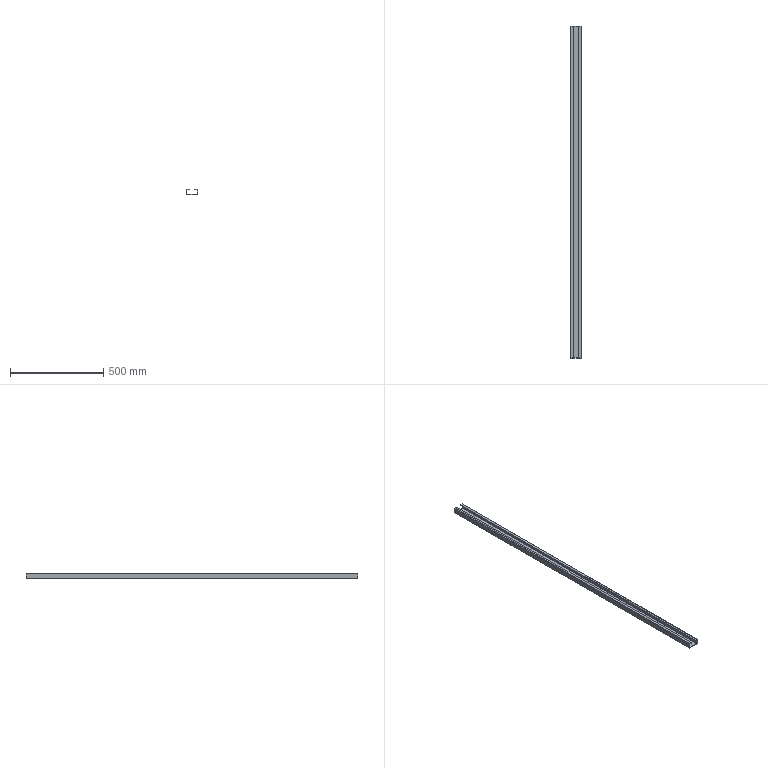Part | SolidWorks | features BaseBody 1 | 1 solid | 38 faces | box 60 x 1776 x 30 mm | volume 606457 mm3 | plane 30 | cylinder 8 | commonest cylinder face diameters 1.473 x4 6.473 x4
STEP:
#1=CARTESIAN_POINT('',(15.,888.,25.));
#2=VERTEX_POINT('',#1);
#3=CARTESIAN_POINT('',(15.,-888.,25.));
#4=VERTEX_POINT('',#3);
#5=CARTESIAN_POINT('',(15.,-888.,25.));
#6=DIRECTION('',(0.,-1.,0.));
#7=VECTOR('',#6,1000.);
#8=LINE('',#5,#7);
#9=EDGE_CURVE('',#2,#4,#8,.T.);
#10=ORIENTED_EDGE('',*,*,#9,.T.);
#11=CARTESIAN_POINT('',(15.,-888.,27.5));
#12=VERTEX_POINT('',#11);
#13=CARTESIAN_POINT('',(15.,-888.,27.5));
#14=DIRECTION('',(0.,0.,-1.));
#15=VECTOR('',#14,1000.);
#16=LINE('',#13,#15);
#17=EDGE_CURVE('',#12,#4,#16,.T.);
#18=ORIENTED_EDGE('',*,*,#17,.F.);
#19=CARTESIAN_POINT('',(15.,888.,27.5));
#20=VERTEX_POINT('',#19);
#21=CARTESIAN_POINT('',(15.,0.,27.5));
#22=DIRECTION('',(0.,-1.,0.));
#23=VECTOR('',#22,1000.);
#24=LINE('',#21,#23);
#25=EDGE_CURVE('',#20,#12,#24,.T.);
#26=ORIENTED_EDGE('',*,*,#25,.F.);
#27=CARTESIAN_POINT('',(15.,888.,27.5));
#28=DIRECTION('',(0.,0.,-1.));
#29=VECTOR('',#28,1000.);
#30=LINE('',#27,#29);
#31=EDGE_CURVE('',#20,#2,#30,.T.);
#32=ORIENTED_EDGE('',*,*,#31,.T.);
#33=EDGE_LOOP('',(#10,#18,#26,#32));
#34=FACE_OUTER_BOUND('',#33,.T.);
#35=CARTESIAN_POINT('',(15.,-888.,27.5));
#36=DIRECTION('',(1.,0.,0.));
#37=DIRECTION('',(0.,0.,-1.));
#38=AXIS2_PLACEMENT_3D('',#35,#36,#37);
#39=PLANE('',#38);
#40=ADVANCED_FACE('',(#34),#39,.F.);
#41=CARTESIAN_POINT('',(26.763,888.,25.));
#42=VERTEX_POINT('',#41);
#43=CARTESIAN_POINT('',(15.,888.,25.));
#44=DIRECTION('',(-1.,0.,0.));
#45=VECTOR('',#44,1000.);
#46=LINE('',#43,#45);
#47=EDGE_CURVE('',#42,#2,#46,.T.);
#48=ORIENTED_EDGE('',*,*,#47,.F.);
#49=CARTESIAN_POINT('',(26.763,-888.,25.));
#50=VERTEX_POINT('',#49);
#51=CARTESIAN_POINT('',(26.763,-888.,25.));
#52=DIRECTION('',(0.,1.,0.));
#53=VECTOR('',#52,1000.);
#54=LINE('',#51,#53);
#55=EDGE_CURVE('',#50,#42,#54,.T.);
#56=ORIENTED_EDGE('',*,*,#55,.F.);
#57=CARTESIAN_POINT('',(27.5,-888.,25.));
#58=DIRECTION('',(1.,0.,0.));
#59=VECTOR('',#58,1000.);
#60=LINE('',#57,#59);
#61=EDGE_CURVE('',#4,#50,#60,.T.);
#62=ORIENTED_EDGE('',*,*,#61,.F.);
#63=ORIENTED_EDGE('',*,*,#9,.F.);
#64=EDGE_LOOP('',(#48,#56,#62,#63));
#65=FACE_OUTER_BOUND('',#64,.T.);
#66=CARTESIAN_POINT('',(0.,0.,25.));
#67=DIRECTION('',(0.,0.,-1.));
#68=DIRECTION('',(-1.,0.,0.));
#69=AXIS2_PLACEMENT_3D('',#66,#67,#68);
#70=PLANE('',#69);
#71=ADVANCED_FACE('',(#65),#70,.T.);
#72=CARTESIAN_POINT('',(26.763,888.,27.5));
#73=VERTEX_POINT('',#72);
#74=CARTESIAN_POINT('',(26.763,-888.,27.5));
#75=VERTEX_POINT('',#74);
#76=CARTESIAN_POINT('',(26.763,-888.,27.5));
#77=DIRECTION('',(0.,-1.,0.));
#78=VECTOR('',#77,1000.);
#79=LINE('',#76,#78);
#80=EDGE_CURVE('',#73,#75,#79,.T.);
#81=ORIENTED_EDGE('',*,*,#80,.F.);
#82=CARTESIAN_POINT('',(0.,888.,27.5));
#83=DIRECTION('',(-1.,0.,0.));
#84=VECTOR('',#83,1000.);
#85=LINE('',#82,#84);
#86=EDGE_CURVE('',#73,#20,#85,.T.);
#87=ORIENTED_EDGE('',*,*,#86,.T.);
#88=ORIENTED_EDGE('',*,*,#25,.T.);
#89=CARTESIAN_POINT('',(0.,-888.,27.5));
#90=DIRECTION('',(1.,0.,0.));
#91=VECTOR('',#90,1000.);
#92=LINE('',#89,#91);
#93=EDGE_CURVE('',#12,#75,#92,.T.);
#94=ORIENTED_EDGE('',*,*,#93,.T.);
#95=EDGE_LOOP('',(#81,#87,#88,#94));
#96=FACE_OUTER_BOUND('',#95,.T.);
#97=CARTESIAN_POINT('',(0.,0.,27.5));
#98=DIRECTION('',(0.,0.,-1.));
#99=DIRECTION('',(-1.,0.,0.));
#100=AXIS2_PLACEMENT_3D('',#97,#98,#99);
#101=PLANE('',#100);
#102=ADVANCED_FACE('',(#96),#101,.F.);
#103=CARTESIAN_POINT('',(26.763,-888.,27.5));
#104=DIRECTION('',(0.,0.,1.));
#105=VECTOR('',#104,1000.);
#106=LINE('',#103,#105);
#107=EDGE_CURVE('',#50,#75,#106,.T.);
#108=ORIENTED_EDGE('',*,*,#107,.T.);
#109=ORIENTED_EDGE('',*,*,#93,.F.);
#110=ORIENTED_EDGE('',*,*,#17,.T.);
#111=ORIENTED_EDGE('',*,*,#61,.T.);
#112=EDGE_LOOP('',(#108,#109,#110,#111));
#113=FACE_OUTER_BOUND('',#112,.T.);
#114=CARTESIAN_POINT('',(27.5,-888.,27.5));
#115=DIRECTION('',(0.,1.,0.));
#116=DIRECTION('',(0.,0.,-1.));
#117=AXIS2_PLACEMENT_3D('',#114,#115,#116);
#118=PLANE('',#117);
#119=ADVANCED_FACE('',(#113),#118,.F.);
#120=CARTESIAN_POINT('',(26.763,888.,25.));
#121=DIRECTION('',(0.,0.,1.));
#122=VECTOR('',#121,1000.);
#123=LINE('',#120,#122);
#124=EDGE_CURVE('',#42,#73,#123,.T.);
#125=ORIENTED_EDGE('',*,*,#124,.F.);
#126=ORIENTED_EDGE('',*,*,#47,.T.);
#127=ORIENTED_EDGE('',*,*,#31,.F.);
#128=ORIENTED_EDGE('',*,*,#86,.F.);
#129=EDGE_LOOP('',(#125,#126,#127,#128));
#130=FACE_OUTER_BOUND('',#129,.T.);
#131=CARTESIAN_POINT('',(15.,888.,27.5));
#132=DIRECTION('',(0.,-1.,0.));
#133=DIRECTION('',(-1.,0.,0.));
#134=AXIS2_PLACEMENT_3D('',#131,#132,#133);
#135=PLANE('',#134);
#136=ADVANCED_FACE('',(#130),#135,.F.);
#137=CARTESIAN_POINT('',(27.5,888.,24.263));
#138=VERTEX_POINT('',#137);
#139=CARTESIAN_POINT('',(27.5,-888.,24.263));
#140=VERTEX_POINT('',#139);
#141=CARTESIAN_POINT('',(27.5,888.,24.263));
#142=DIRECTION('',(0.,-1.,0.));
#143=VECTOR('',#142,1000.);
#144=LINE('',#141,#143);
#145=EDGE_CURVE('',#138,#140,#144,.T.);
#146=ORIENTED_EDGE('',*,*,#145,.T.);
#147=CARTESIAN_POINT('',(26.763,-888.,24.263));
#148=DIRECTION('',(0.,-1.,0.));
#149=DIRECTION('',(0.,0.,1.));
#150=AXIS2_PLACEMENT_3D('',#147,#148,#149);
#151=CIRCLE('',#150,0.7366);
#152=EDGE_CURVE('',#140,#50,#151,.T.);
#153=ORIENTED_EDGE('',*,*,#152,.T.);
#154=ORIENTED_EDGE('',*,*,#55,.T.);
#155=CARTESIAN_POINT('',(26.763,888.,24.263));
#156=DIRECTION('',(0.,1.,0.));
#157=DIRECTION('',(0.,0.,1.));
#158=AXIS2_PLACEMENT_3D('',#155,#156,#157);
#159=CIRCLE('',#158,0.7366);
#160=EDGE_CURVE('',#42,#138,#159,.T.);
#161=ORIENTED_EDGE('',*,*,#160,.T.);
#162=EDGE_LOOP('',(#146,#153,#154,#161));
#163=FACE_OUTER_BOUND('',#162,.T.);
#164=CARTESIAN_POINT('',(26.763,888.,24.263));
#165=DIRECTION('',(0.,1.,0.));
#166=DIRECTION('',(0.,0.,1.));
#167=AXIS2_PLACEMENT_3D('',#164,#165,#166);
#168=CYLINDRICAL_SURFACE('',#167,0.7366);
#169=ADVANCED_FACE('',(#163),#168,.F.);
#170=CARTESIAN_POINT('',(30.,888.,24.263));
#171=VERTEX_POINT('',#170);
#172=CARTESIAN_POINT('',(30.,-888.,24.263));
#173=VERTEX_POINT('',#172);
#174=CARTESIAN_POINT('',(30.,888.,24.263));
#175=DIRECTION('',(0.,-1.,0.));
#176=VECTOR('',#175,1000.);
#177=LINE('',#174,#176);
#178=EDGE_CURVE('',#171,#173,#177,.T.);
#179=ORIENTED_EDGE('',*,*,#178,.F.);
#180=CARTESIAN_POINT('',(26.763,888.,24.263));
#181=DIRECTION('',(0.,1.,0.));
#182=DIRECTION('',(0.,0.,1.));
#183=AXIS2_PLACEMENT_3D('',#180,#181,#182);
#184=CIRCLE('',#183,3.237);
#185=EDGE_CURVE('',#73,#171,#184,.T.);
#186=ORIENTED_EDGE('',*,*,#185,.F.);
#187=ORIENTED_EDGE('',*,*,#80,.T.);
#188=CARTESIAN_POINT('',(26.763,-888.,24.263));
#189=DIRECTION('',(0.,-1.,0.));
#190=DIRECTION('',(0.,0.,1.));
#191=AXIS2_PLACEMENT_3D('',#188,#189,#190);
#192=CIRCLE('',#191,3.237);
#193=EDGE_CURVE('',#173,#75,#192,.T.);
#194=ORIENTED_EDGE('',*,*,#193,.F.);
#195=EDGE_LOOP('',(#179,#186,#187,#194));
#196=FACE_OUTER_BOUND('',#195,.T.);
#197=CARTESIAN_POINT('',(26.763,888.,24.263));
#198=DIRECTION('',(0.,1.,0.));
#199=DIRECTION('',(0.,0.,1.));
#200=AXIS2_PLACEMENT_3D('',#197,#198,#199);
#201=CYLINDRICAL_SURFACE('',#200,3.237);
#202=ADVANCED_FACE('',(#196),#201,.T.);
#203=ORIENTED_EDGE('',*,*,#160,.F.);
#204=ORIENTED_EDGE('',*,*,#124,.T.);
#205=ORIENTED_EDGE('',*,*,#185,.T.);
#206=CARTESIAN_POINT('',(27.5,888.,24.263));
#207=DIRECTION('',(1.,0.,0.));
#208=VECTOR('',#207,1000.);
#209=LINE('',#206,#208);
#210=EDGE_CURVE('',#138,#171,#209,.T.);
#211=ORIENTED_EDGE('',*,*,#210,.F.);
#212=EDGE_LOOP('',(#203,#204,#205,#211));
#213=FACE_OUTER_BOUND('',#212,.T.);
#214=CARTESIAN_POINT('',(26.763,888.,24.263));
#215=DIRECTION('',(0.,-1.,0.));
#216=DIRECTION('',(0.,0.,-1.));
#217=AXIS2_PLACEMENT_3D('',#214,#215,#216);
#218=PLANE('',#217);
#219=ADVANCED_FACE('',(#213),#218,.F.);
#220=ORIENTED_EDGE('',*,*,#107,.F.);
#221=ORIENTED_EDGE('',*,*,#152,.F.);
#222=CARTESIAN_POINT('',(27.5,-888.,24.263));
#223=DIRECTION('',(1.,0.,0.));
#224=VECTOR('',#223,1000.);
#225=LINE('',#222,#224);
#226=EDGE_CURVE('',#140,#173,#225,.T.);
#227=ORIENTED_EDGE('',*,*,#226,.T.);
#228=ORIENTED_EDGE('',*,*,#193,.T.);
#229=EDGE_LOOP('',(#220,#221,#227,#228));
#230=FACE_OUTER_BOUND('',#229,.T.);
#231=CARTESIAN_POINT('',(26.763,-888.,24.263));
#232=DIRECTION('',(0.,-1.,0.));
#233=DIRECTION('',(0.,0.,-1.));
#234=AXIS2_PLACEMENT_3D('',#231,#232,#233);
#235=PLANE('',#234);
#236=ADVANCED_FACE('',(#230),#235,.T.);
#237=CARTESIAN_POINT('',(-15.,-888.,25.));
#238=VERTEX_POINT('',#237);
#239=CARTESIAN_POINT('',(-15.,888.,25.));
#240=VERTEX_POINT('',#239);
#241=CARTESIAN_POINT('',(-15.,888.,25.));
#242=DIRECTION('',(0.,1.,0.));
#243=VECTOR('',#242,1000.);
#244=LINE('',#241,#243);
#245=EDGE_CURVE('',#238,#240,#244,.T.);
#246=ORIENTED_EDGE('',*,*,#245,.T.);
#247=CARTESIAN_POINT('',(-15.,888.,27.5));
#248=VERTEX_POINT('',#247);
#249=CARTESIAN_POINT('',(-15.,888.,27.5));
#250=DIRECTION('',(0.,0.,-1.));
#251=VECTOR('',#250,1000.);
#252=LINE('',#249,#251);
#253=EDGE_CURVE('',#248,#240,#252,.T.);
#254=ORIENTED_EDGE('',*,*,#253,.F.);
#255=CARTESIAN_POINT('',(-15.,-888.,27.5));
#256=VERTEX_POINT('',#255);
#257=CARTESIAN_POINT('',(-15.,0.,27.5));
#258=DIRECTION('',(0.,1.,0.));
#259=VECTOR('',#258,1000.);
#260=LINE('',#257,#259);
#261=EDGE_CURVE('',#256,#248,#260,.T.);
#262=ORIENTED_EDGE('',*,*,#261,.F.);
#263=CARTESIAN_POINT('',(-15.,-888.,27.5));
#264=DIRECTION('',(0.,0.,-1.));
#265=VECTOR('',#264,1000.);
#266=LINE('',#263,#265);
#267=EDGE_CURVE('',#256,#238,#266,.T.);
#268=ORIENTED_EDGE('',*,*,#267,.T.);
#269=EDGE_LOOP('',(#246,#254,#262,#268));
#270=FACE_OUTER_BOUND('',#269,.T.);
#271=CARTESIAN_POINT('',(-15.,888.,27.5));
#272=DIRECTION('',(-1.,0.,0.));
#273=DIRECTION('',(0.,0.,1.));
#274=AXIS2_PLACEMENT_3D('',#271,#272,#273);
#275=PLANE('',#274);
#276=ADVANCED_FACE('',(#270),#275,.F.);
#277=CARTESIAN_POINT('',(-26.763,-888.,25.));
#278=VERTEX_POINT('',#277);
#279=CARTESIAN_POINT('',(-15.,-888.,25.));
#280=DIRECTION('',(1.,0.,0.));
#281=VECTOR('',#280,1000.);
#282=LINE('',#279,#281);
#283=EDGE_CURVE('',#278,#238,#282,.T.);
#284=ORIENTED_EDGE('',*,*,#283,.F.);
#285=CARTESIAN_POINT('',(-26.763,888.,25.));
#286=VERTEX_POINT('',#285);
#287=CARTESIAN_POINT('',(-26.763,888.,25.));
#288=DIRECTION('',(0.,-1.,0.));
#289=VECTOR('',#288,1000.);
#290=LINE('',#287,#289);
#291=EDGE_CURVE('',#286,#278,#290,.T.);
#292=ORIENTED_EDGE('',*,*,#291,.F.);
#293=CARTESIAN_POINT('',(-27.5,888.,25.));
#294=DIRECTION('',(-1.,0.,0.));
#295=VECTOR('',#294,1000.);
#296=LINE('',#293,#295);
#297=EDGE_CURVE('',#240,#286,#296,.T.);
#298=ORIENTED_EDGE('',*,*,#297,.F.);
#299=ORIENTED_EDGE('',*,*,#245,.F.);
#300=EDGE_LOOP('',(#284,#292,#298,#299));
#301=FACE_OUTER_BOUND('',#300,.T.);
#302=CARTESIAN_POINT('',(0.,0.,25.));
#303=DIRECTION('',(0.,0.,-1.));
#304=DIRECTION('',(0.,-1.,0.));
#305=AXIS2_PLACEMENT_3D('',#302,#303,#304);
#306=PLANE('',#305);
#307=ADVANCED_FACE('',(#301),#306,.T.);
#308=CARTESIAN_POINT('',(-26.763,-888.,27.5));
#309=VERTEX_POINT('',#308);
#310=CARTESIAN_POINT('',(-26.763,888.,27.5));
#311=VERTEX_POINT('',#310);
#312=CARTESIAN_POINT('',(-26.763,888.,27.5));
#313=DIRECTION('',(0.,1.,0.));
#314=VECTOR('',#313,1000.);
#315=LINE('',#312,#314);
#316=EDGE_CURVE('',#309,#311,#315,.T.);
#317=ORIENTED_EDGE('',*,*,#316,.F.);
#318=CARTESIAN_POINT('',(0.,-888.,27.5));
#319=DIRECTION('',(1.,0.,0.));
#320=VECTOR('',#319,1000.);
#321=LINE('',#318,#320);
#322=EDGE_CURVE('',#309,#256,#321,.T.);
#323=ORIENTED_EDGE('',*,*,#322,.T.);
#324=ORIENTED_EDGE('',*,*,#261,.T.);
#325=CARTESIAN_POINT('',(0.,888.,27.5));
#326=DIRECTION('',(-1.,0.,0.));
#327=VECTOR('',#326,1000.);
#328=LINE('',#325,#327);
#329=EDGE_CURVE('',#248,#311,#328,.T.);
#330=ORIENTED_EDGE('',*,*,#329,.T.);
#331=EDGE_LOOP('',(#317,#323,#324,#330));
#332=FACE_OUTER_BOUND('',#331,.T.);
#333=CARTESIAN_POINT('',(0.,0.,27.5));
#334=DIRECTION('',(0.,0.,-1.));
#335=DIRECTION('',(0.,-1.,0.));
#336=AXIS2_PLACEMENT_3D('',#333,#334,#335);
#337=PLANE('',#336);
#338=ADVANCED_FACE('',(#332),#337,.F.);
#339=CARTESIAN_POINT('',(-26.763,888.,27.5));
#340=DIRECTION('',(0.,0.,1.));
#341=VECTOR('',#340,1000.);
#342=LINE('',#339,#341);
#343=EDGE_CURVE('',#286,#311,#342,.T.);
#344=ORIENTED_EDGE('',*,*,#343,.T.);
#345=ORIENTED_EDGE('',*,*,#329,.F.);
#346=ORIENTED_EDGE('',*,*,#253,.T.);
#347=ORIENTED_EDGE('',*,*,#297,.T.);
#348=EDGE_LOOP('',(#344,#345,#346,#347));
#349=FACE_OUTER_BOUND('',#348,.T.);
#350=CARTESIAN_POINT('',(-27.5,888.,27.5));
#351=DIRECTION('',(0.,-1.,0.));
#352=DIRECTION('',(0.,0.,-1.));
#353=AXIS2_PLACEMENT_3D('',#350,#351,#352);
#354=PLANE('',#353);
#355=ADVANCED_FACE('',(#349),#354,.F.);
#356=CARTESIAN_POINT('',(-26.763,-888.,25.));
#357=DIRECTION('',(0.,0.,1.));
#358=VECTOR('',#357,1000.);
#359=LINE('',#356,#358);
#360=EDGE_CURVE('',#278,#309,#359,.T.);
#361=ORIENTED_EDGE('',*,*,#360,.F.);
#362=ORIENTED_EDGE('',*,*,#283,.T.);
#363=ORIENTED_EDGE('',*,*,#267,.F.);
#364=ORIENTED_EDGE('',*,*,#322,.F.);
#365=EDGE_LOOP('',(#361,#362,#363,#364));
#366=FACE_OUTER_BOUND('',#365,.T.);
#367=CARTESIAN_POINT('',(-15.,-888.,27.5));
#368=DIRECTION('',(0.,1.,0.));
#369=DIRECTION('',(0.,0.,-1.));
#370=AXIS2_PLACEMENT_3D('',#367,#368,#369);
#371=PLANE('',#370);
#372=ADVANCED_FACE('',(#366),#371,.F.);
#373=CARTESIAN_POINT('',(-27.5,-888.,24.263));
#374=VERTEX_POINT('',#373);
#375=CARTESIAN_POINT('',(-27.5,888.,24.263));
#376=VERTEX_POINT('',#375);
#377=CARTESIAN_POINT('',(-27.5,-888.,24.263));
#378=DIRECTION('',(0.,1.,0.));
#379=VECTOR('',#378,1000.);
#380=LINE('',#377,#379);
#381=EDGE_CURVE('',#374,#376,#380,.T.);
#382=ORIENTED_EDGE('',*,*,#381,.T.);
#383=CARTESIAN_POINT('',(-26.763,888.,24.263));
#384=DIRECTION('',(0.,1.,0.));
#385=DIRECTION('',(0.,0.,-1.));
#386=AXIS2_PLACEMENT_3D('',#383,#384,#385);
#387=CIRCLE('',#386,0.7366);
#388=EDGE_CURVE('',#376,#286,#387,.T.);
#389=ORIENTED_EDGE('',*,*,#388,.T.);
#390=ORIENTED_EDGE('',*,*,#291,.T.);
#391=CARTESIAN_POINT('',(-26.763,-888.,24.263));
#392=DIRECTION('',(0.,-1.,0.));
#393=DIRECTION('',(0.,0.,-1.));
#394=AXIS2_PLACEMENT_3D('',#391,#392,#393);
#395=CIRCLE('',#394,0.7366);
#396=EDGE_CURVE('',#278,#374,#395,.T.);
#397=ORIENTED_EDGE('',*,*,#396,.T.);
#398=EDGE_LOOP('',(#382,#389,#390,#397));
#399=FACE_OUTER_BOUND('',#398,.T.);
#400=CARTESIAN_POINT('',(-26.763,-888.,24.263));
#401=DIRECTION('',(0.,-1.,0.));
#402=DIRECTION('',(0.,0.,1.));
#403=AXIS2_PLACEMENT_3D('',#400,#401,#402);
#404=CYLINDRICAL_SURFACE('',#403,0.7366);
#405=ADVANCED_FACE('',(#399),#404,.F.);
#406=CARTESIAN_POINT('',(-30.,-888.,24.263));
#407=VERTEX_POINT('',#406);
#408=CARTESIAN_POINT('',(-30.,888.,24.263));
#409=VERTEX_POINT('',#408);
#410=CARTESIAN_POINT('',(-30.,-888.,24.263));
#411=DIRECTION('',(0.,1.,0.));
#412=VECTOR('',#411,1000.);
#413=LINE('',#410,#412);
#414=EDGE_CURVE('',#407,#409,#413,.T.);
#415=ORIENTED_EDGE('',*,*,#414,.F.);
#416=CARTESIAN_POINT('',(-26.763,-888.,24.263));
#417=DIRECTION('',(0.,-1.,0.));
#418=DIRECTION('',(0.,0.,-1.));
#419=AXIS2_PLACEMENT_3D('',#416,#417,#418);
#420=CIRCLE('',#419,3.237);
#421=EDGE_CURVE('',#309,#407,#420,.T.);
#422=ORIENTED_EDGE('',*,*,#421,.F.);
#423=ORIENTED_EDGE('',*,*,#316,.T.);
#424=CARTESIAN_POINT('',(-26.763,888.,24.263));
#425=DIRECTION('',(0.,1.,0.));
#426=DIRECTION('',(0.,0.,-1.));
#427=AXIS2_PLACEMENT_3D('',#424,#425,#426);
#428=CIRCLE('',#427,3.237);
#429=EDGE_CURVE('',#409,#311,#428,.T.);
#430=ORIENTED_EDGE('',*,*,#429,.F.);
#431=EDGE_LOOP('',(#415,#422,#423,#430));
#432=FACE_OUTER_BOUND('',#431,.T.);
#433=CARTESIAN_POINT('',(-26.763,-888.,24.263));
#434=DIRECTION('',(0.,-1.,0.));
#435=DIRECTION('',(0.,0.,1.));
#436=AXIS2_PLACEMENT_3D('',#433,#434,#435);
#437=CYLINDRICAL_SURFACE('',#436,3.237);
#438=ADVANCED_FACE('',(#432),#437,.T.);
#439=ORIENTED_EDGE('',*,*,#396,.F.);
#440=ORIENTED_EDGE('',*,*,#360,.T.);
#441=ORIENTED_EDGE('',*,*,#421,.T.);
#442=CARTESIAN_POINT('',(-27.5,-888.,24.263));
#443=DIRECTION('',(-1.,0.,0.));
#444=VECTOR('',#443,1000.);
#445=LINE('',#442,#444);
#446=EDGE_CURVE('',#374,#407,#445,.T.);
#447=ORIENTED_EDGE('',*,*,#446,.F.);
#448=EDGE_LOOP('',(#439,#440,#441,#447));
#449=FACE_OUTER_BOUND('',#448,.T.);
#450=CARTESIAN_POINT('',(-26.763,-888.,24.263));
#451=DIRECTION('',(0.,1.,0.));
#452=DIRECTION('',(1.,0.,0.));
#453=AXIS2_PLACEMENT_3D('',#450,#451,#452);
#454=PLANE('',#453);
#455=ADVANCED_FACE('',(#449),#454,.F.);
#456=ORIENTED_EDGE('',*,*,#343,.F.);
#457=ORIENTED_EDGE('',*,*,#388,.F.);
#458=CARTESIAN_POINT('',(-27.5,888.,24.263));
#459=DIRECTION('',(-1.,0.,0.));
#460=VECTOR('',#459,1000.);
#461=LINE('',#458,#460);
#462=EDGE_CURVE('',#376,#409,#461,.T.);
#463=ORIENTED_EDGE('',*,*,#462,.T.);
#464=ORIENTED_EDGE('',*,*,#429,.T.);
#465=EDGE_LOOP('',(#456,#457,#463,#464));
#466=FACE_OUTER_BOUND('',#465,.T.);
#467=CARTESIAN_POINT('',(-26.763,888.,24.263));
#468=DIRECTION('',(0.,1.,0.));
#469=DIRECTION('',(1.,0.,0.));
#470=AXIS2_PLACEMENT_3D('',#467,#468,#469);
#471=PLANE('',#470);
#472=ADVANCED_FACE('',(#466),#471,.T.);
#473=CARTESIAN_POINT('',(26.763,888.,0.));
#474=VERTEX_POINT('',#473);
#475=CARTESIAN_POINT('',(26.763,-888.,0.));
#476=VERTEX_POINT('',#475);
#477=CARTESIAN_POINT('',(26.763,888.,0.));
#478=DIRECTION('',(0.,-1.,0.));
#479=VECTOR('',#478,1000.);
#480=LINE('',#477,#479);
#481=EDGE_CURVE('',#474,#476,#480,.T.);
#482=ORIENTED_EDGE('',*,*,#481,.T.);
#483=CARTESIAN_POINT('',(27.5,-888.,0.7366));
#484=VERTEX_POINT('',#483);
#485=CARTESIAN_POINT('',(26.763,-888.,0.7366));
#486=DIRECTION('',(0.,-1.,0.));
#487=DIRECTION('',(0.,0.,1.));
#488=AXIS2_PLACEMENT_3D('',#485,#486,#487);
#489=CIRCLE('',#488,0.7366);
#490=EDGE_CURVE('',#476,#484,#489,.T.);
#491=ORIENTED_EDGE('',*,*,#490,.T.);
#492=CARTESIAN_POINT('',(27.5,888.,0.7366));
#493=VERTEX_POINT('',#492);
#494=CARTESIAN_POINT('',(27.5,-888.,0.7366));
#495=DIRECTION('',(0.,1.,0.));
#496=VECTOR('',#495,1000.);
#497=LINE('',#494,#496);
#498=EDGE_CURVE('',#484,#493,#497,.T.);
#499=ORIENTED_EDGE('',*,*,#498,.T.);
#500=CARTESIAN_POINT('',(26.763,888.,0.7366));
#501=DIRECTION('',(0.,1.,0.));
#502=DIRECTION('',(0.,0.,1.));
#503=AXIS2_PLACEMENT_3D('',#500,#501,#502);
#504=CIRCLE('',#503,0.7366);
#505=EDGE_CURVE('',#493,#474,#504,.T.);
#506=ORIENTED_EDGE('',*,*,#505,.T.);
#507=EDGE_LOOP('',(#482,#491,#499,#506));
#508=FACE_OUTER_BOUND('',#507,.T.);
#509=CARTESIAN_POINT('',(26.763,888.,0.7366));
#510=DIRECTION('',(0.,1.,0.));
#511=DIRECTION('',(1.,0.,0.));
#512=AXIS2_PLACEMENT_3D('',#509,#510,#511);
#513=CYLINDRICAL_SURFACE('',#512,0.7366);
#514=ADVANCED_FACE('',(#508),#513,.F.);
#515=CARTESIAN_POINT('',(26.763,888.,-2.5));
#516=VERTEX_POINT('',#515);
#517=CARTESIAN_POINT('',(26.763,-888.,-2.5));
#518=VERTEX_POINT('',#517);
#519=CARTESIAN_POINT('',(26.763,888.,-2.5));
#520=DIRECTION('',(0.,-1.,0.));
#521=VECTOR('',#520,1000.);
#522=LINE('',#519,#521);
#523=EDGE_CURVE('',#516,#518,#522,.T.);
#524=ORIENTED_EDGE('',*,*,#523,.F.);
#525=CARTESIAN_POINT('',(30.,888.,0.7366));
#526=VERTEX_POINT('',#525);
#527=CARTESIAN_POINT('',(26.763,888.,0.7366));
#528=DIRECTION('',(0.,1.,0.));
#529=DIRECTION('',(0.,0.,1.));
#530=AXIS2_PLACEMENT_3D('',#527,#528,#529);
#531=CIRCLE('',#530,3.237);
#532=EDGE_CURVE('',#526,#516,#531,.T.);
#533=ORIENTED_EDGE('',*,*,#532,.F.);
#534=CARTESIAN_POINT('',(30.,-888.,0.7366));
#535=VERTEX_POINT('',#534);
#536=CARTESIAN_POINT('',(30.,-888.,0.7366));
#537=DIRECTION('',(0.,-1.,0.));
#538=VECTOR('',#537,1000.);
#539=LINE('',#536,#538);
#540=EDGE_CURVE('',#526,#535,#539,.T.);
#541=ORIENTED_EDGE('',*,*,#540,.T.);
#542=CARTESIAN_POINT('',(26.763,-888.,0.7366));
#543=DIRECTION('',(0.,-1.,0.));
#544=DIRECTION('',(0.,0.,1.));
#545=AXIS2_PLACEMENT_3D('',#542,#543,#544);
#546=CIRCLE('',#545,3.237);
#547=EDGE_CURVE('',#518,#535,#546,.T.);
#548=ORIENTED_EDGE('',*,*,#547,.F.);
#549=EDGE_LOOP('',(#524,#533,#541,#548));
#550=FACE_OUTER_BOUND('',#549,.T.);
#551=CARTESIAN_POINT('',(26.763,888.,0.7366));
#552=DIRECTION('',(0.,1.,0.));
#553=DIRECTION('',(1.,0.,0.));
#554=AXIS2_PLACEMENT_3D('',#551,#552,#553);
#555=CYLINDRICAL_SURFACE('',#554,3.237);
#556=ADVANCED_FACE('',(#550),#555,.T.);
#557=ORIENTED_EDGE('',*,*,#505,.F.);
#558=CARTESIAN_POINT('',(27.5,888.,0.7366));
#559=DIRECTION('',(1.,0.,0.));
#560=VECTOR('',#559,1000.);
#561=LINE('',#558,#560);
#562=EDGE_CURVE('',#493,#526,#561,.T.);
#563=ORIENTED_EDGE('',*,*,#562,.T.);
#564=ORIENTED_EDGE('',*,*,#532,.T.);
#565=CARTESIAN_POINT('',(26.763,888.,0.));
#566=DIRECTION('',(0.,0.,-1.));
#567=VECTOR('',#566,1000.);
#568=LINE('',#565,#567);
#569=EDGE_CURVE('',#474,#516,#568,.T.);
#570=ORIENTED_EDGE('',*,*,#569,.F.);
#571=EDGE_LOOP('',(#557,#563,#564,#570));
#572=FACE_OUTER_BOUND('',#571,.T.);
#573=CARTESIAN_POINT('',(26.763,888.,0.7366));
#574=DIRECTION('',(0.,-1.,0.));
#575=DIRECTION('',(0.,0.,-1.));
#576=AXIS2_PLACEMENT_3D('',#573,#574,#575);
#577=PLANE('',#576);
#578=ADVANCED_FACE('',(#572),#577,.F.);
#579=CARTESIAN_POINT('',(30.,-888.,0.7366));
#580=DIRECTION('',(1.,0.,0.));
#581=VECTOR('',#580,1000.);
#582=LINE('',#579,#581);
#583=EDGE_CURVE('',#484,#535,#582,.T.);
#584=ORIENTED_EDGE('',*,*,#583,.F.);
#585=ORIENTED_EDGE('',*,*,#490,.F.);
#586=CARTESIAN_POINT('',(26.763,-888.,0.));
#587=DIRECTION('',(0.,0.,-1.));
#588=VECTOR('',#587,1000.);
#589=LINE('',#586,#588);
#590=EDGE_CURVE('',#476,#518,#589,.T.);
#591=ORIENTED_EDGE('',*,*,#590,.T.);
#592=ORIENTED_EDGE('',*,*,#547,.T.);
#593=EDGE_LOOP('',(#584,#585,#591,#592));
#594=FACE_OUTER_BOUND('',#593,.T.);
#595=CARTESIAN_POINT('',(26.763,-888.,0.7366));
#596=DIRECTION('',(0.,-1.,0.));
#597=DIRECTION('',(0.,0.,-1.));
#598=AXIS2_PLACEMENT_3D('',#595,#596,#597);
#599=PLANE('',#598);
#600=ADVANCED_FACE('',(#594),#599,.T.);
#601=CARTESIAN_POINT('',(-26.763,-888.,0.));
#602=VERTEX_POINT('',#601);
#603=CARTESIAN_POINT('',(-26.763,888.,0.));
#604=VERTEX_POINT('',#603);
#605=CARTESIAN_POINT('',(-26.763,-888.,0.));
#606=DIRECTION('',(0.,1.,0.));
#607=VECTOR('',#606,1000.);
#608=LINE('',#605,#607);
#609=EDGE_CURVE('',#602,#604,#608,.T.);
#610=ORIENTED_EDGE('',*,*,#609,.T.);
#611=CARTESIAN_POINT('',(-27.5,888.,0.7366));
#612=VERTEX_POINT('',#611);
#613=CARTESIAN_POINT('',(-26.763,888.,0.7366));
#614=DIRECTION('',(0.,1.,0.));
#615=DIRECTION('',(0.,0.,-1.));
#616=AXIS2_PLACEMENT_3D('',#613,#614,#615);
#617=CIRCLE('',#616,0.7366);
#618=EDGE_CURVE('',#604,#612,#617,.T.);
#619=ORIENTED_EDGE('',*,*,#618,.T.);
#620=CARTESIAN_POINT('',(-27.5,-888.,0.7366));
#621=VERTEX_POINT('',#620);
#622=CARTESIAN_POINT('',(-27.5,888.,0.7366));
#623=DIRECTION('',(0.,-1.,0.));
#624=VECTOR('',#623,1000.);
#625=LINE('',#622,#624);
#626=EDGE_CURVE('',#612,#621,#625,.T.);
#627=ORIENTED_EDGE('',*,*,#626,.T.);
#628=CARTESIAN_POINT('',(-26.763,-888.,0.7366));
#629=DIRECTION('',(0.,-1.,0.));
#630=DIRECTION('',(0.,0.,-1.));
#631=AXIS2_PLACEMENT_3D('',#628,#629,#630);
#632=CIRCLE('',#631,0.7366);
#633=EDGE_CURVE('',#621,#602,#632,.T.);
#634=ORIENTED_EDGE('',*,*,#633,.T.);
#635=EDGE_LOOP('',(#610,#619,#627,#634));
#636=FACE_OUTER_BOUND('',#635,.T.);
#637=CARTESIAN_POINT('',(-26.763,-888.,0.7366));
#638=DIRECTION('',(0.,-1.,0.));
#639=DIRECTION('',(-1.,0.,0.));
#640=AXIS2_PLACEMENT_3D('',#637,#638,#639);
#641=CYLINDRICAL_SURFACE('',#640,0.7366);
#642=ADVANCED_FACE('',(#636),#641,.F.);
#643=CARTESIAN_POINT('',(-26.763,-888.,-2.5));
#644=VERTEX_POINT('',#643);
#645=CARTESIAN_POINT('',(-26.763,888.,-2.5));
#646=VERTEX_POINT('',#645);
#647=CARTESIAN_POINT('',(-26.763,-888.,-2.5));
#648=DIRECTION('',(0.,1.,0.));
#649=VECTOR('',#648,1000.);
#650=LINE('',#647,#649);
#651=EDGE_CURVE('',#644,#646,#650,.T.);
#652=ORIENTED_EDGE('',*,*,#651,.F.);
#653=CARTESIAN_POINT('',(-30.,-888.,0.7366));
#654=VERTEX_POINT('',#653);
#655=CARTESIAN_POINT('',(-26.763,-888.,0.7366));
#656=DIRECTION('',(0.,-1.,0.));
#657=DIRECTION('',(0.,0.,-1.));
#658=AXIS2_PLACEMENT_3D('',#655,#656,#657);
#659=CIRCLE('',#658,3.237);
#660=EDGE_CURVE('',#654,#644,#659,.T.);
#661=ORIENTED_EDGE('',*,*,#660,.F.);
#662=CARTESIAN_POINT('',(-30.,888.,0.7366));
#663=VERTEX_POINT('',#662);
#664=CARTESIAN_POINT('',(-30.,888.,0.7366));
#665=DIRECTION('',(0.,1.,0.));
#666=VECTOR('',#665,1000.);
#667=LINE('',#664,#666);
#668=EDGE_CURVE('',#654,#663,#667,.T.);
#669=ORIENTED_EDGE('',*,*,#668,.T.);
#670=CARTESIAN_POINT('',(-26.763,888.,0.7366));
#671=DIRECTION('',(0.,1.,0.));
#672=DIRECTION('',(0.,0.,-1.));
#673=AXIS2_PLACEMENT_3D('',#670,#671,#672);
#674=CIRCLE('',#673,3.237);
#675=EDGE_CURVE('',#646,#663,#674,.T.);
#676=ORIENTED_EDGE('',*,*,#675,.F.);
#677=EDGE_LOOP('',(#652,#661,#669,#676));
#678=FACE_OUTER_BOUND('',#677,.T.);
#679=CARTESIAN_POINT('',(-26.763,-888.,0.7366));
#680=DIRECTION('',(0.,-1.,0.));
#681=DIRECTION('',(-1.,0.,0.));
#682=AXIS2_PLACEMENT_3D('',#679,#680,#681);
#683=CYLINDRICAL_SURFACE('',#682,3.237);
#684=ADVANCED_FACE('',(#678),#683,.T.);
#685=ORIENTED_EDGE('',*,*,#633,.F.);
#686=CARTESIAN_POINT('',(-27.5,-888.,0.7366));
#687=DIRECTION('',(-1.,0.,0.));
#688=VECTOR('',#687,1000.);
#689=LINE('',#686,#688);
#690=EDGE_CURVE('',#621,#654,#689,.T.);
#691=ORIENTED_EDGE('',*,*,#690,.T.);
#692=ORIENTED_EDGE('',*,*,#660,.T.);
#693=CARTESIAN_POINT('',(-26.763,-888.,0.));
#694=DIRECTION('',(0.,0.,-1.));
#695=VECTOR('',#694,1000.);
#696=LINE('',#693,#695);
#697=EDGE_CURVE('',#602,#644,#696,.T.);
#698=ORIENTED_EDGE('',*,*,#697,.F.);
#699=EDGE_LOOP('',(#685,#691,#692,#698));
#700=FACE_OUTER_BOUND('',#699,.T.);
#701=CARTESIAN_POINT('',(-26.763,-888.,0.7366));
#702=DIRECTION('',(0.,1.,0.));
#703=DIRECTION('',(0.,0.,-1.));
#704=AXIS2_PLACEMENT_3D('',#701,#702,#703);
#705=PLANE('',#704);
#706=ADVANCED_FACE('',(#700),#705,.F.);
#707=CARTESIAN_POINT('',(-30.,888.,0.7366));
#708=DIRECTION('',(-1.,0.,0.));
#709=VECTOR('',#708,1000.);
#710=LINE('',#707,#709);
#711=EDGE_CURVE('',#612,#663,#710,.T.);
#712=ORIENTED_EDGE('',*,*,#711,.F.);
#713=ORIENTED_EDGE('',*,*,#618,.F.);
#714=CARTESIAN_POINT('',(-26.763,888.,0.));
#715=DIRECTION('',(0.,0.,-1.));
#716=VECTOR('',#715,1000.);
#717=LINE('',#714,#716);
#718=EDGE_CURVE('',#604,#646,#717,.T.);
#719=ORIENTED_EDGE('',*,*,#718,.T.);
#720=ORIENTED_EDGE('',*,*,#675,.T.);
#721=EDGE_LOOP('',(#712,#713,#719,#720));
#722=FACE_OUTER_BOUND('',#721,.T.);
#723=CARTESIAN_POINT('',(-26.763,888.,0.7366));
#724=DIRECTION('',(0.,1.,0.));
#725=DIRECTION('',(0.,0.,-1.));
#726=AXIS2_PLACEMENT_3D('',#723,#724,#725);
#727=PLANE('',#726);
#728=ADVANCED_FACE('',(#722),#727,.T.);
#729=ORIENTED_EDGE('',*,*,#590,.F.);
#730=CARTESIAN_POINT('',(30.,-888.,0.));
#731=DIRECTION('',(1.,0.,0.));
#732=VECTOR('',#731,1000.);
#733=LINE('',#730,#732);
#734=EDGE_CURVE('',#602,#476,#733,.T.);
#735=ORIENTED_EDGE('',*,*,#734,.F.);
#736=ORIENTED_EDGE('',*,*,#697,.T.);
#737=CARTESIAN_POINT('',(30.,-888.,-2.5));
#738=DIRECTION('',(1.,0.,0.));
#739=VECTOR('',#738,1000.);
#740=LINE('',#737,#739);
#741=EDGE_CURVE('',#644,#518,#740,.T.);
#742=ORIENTED_EDGE('',*,*,#741,.T.);
#743=EDGE_LOOP('',(#729,#735,#736,#742));
#744=FACE_OUTER_BOUND('',#743,.T.);
#745=CARTESIAN_POINT('',(30.,-888.,-2.5));
#746=DIRECTION('',(0.,-1.,0.));
#747=DIRECTION('',(0.,0.,-1.));
#748=AXIS2_PLACEMENT_3D('',#745,#746,#747);
#749=PLANE('',#748);
#750=ADVANCED_FACE('',(#744),#749,.T.);
#751=CARTESIAN_POINT('',(30.,888.,0.));
#752=DIRECTION('',(-1.,0.,0.));
#753=VECTOR('',#752,1000.);
#754=LINE('',#751,#753);
#755=EDGE_CURVE('',#474,#604,#754,.T.);
#756=ORIENTED_EDGE('',*,*,#755,.F.);
#757=ORIENTED_EDGE('',*,*,#569,.T.);
#758=CARTESIAN_POINT('',(30.,888.,-2.5));
#759=DIRECTION('',(-1.,0.,0.));
#760=VECTOR('',#759,1000.);
#761=LINE('',#758,#760);
#762=EDGE_CURVE('',#516,#646,#761,.T.);
#763=ORIENTED_EDGE('',*,*,#762,.T.);
#764=ORIENTED_EDGE('',*,*,#718,.F.);
#765=EDGE_LOOP('',(#756,#757,#763,#764));
#766=FACE_OUTER_BOUND('',#765,.T.);
#767=CARTESIAN_POINT('',(30.,888.,-2.5));
#768=DIRECTION('',(0.,1.,0.));
#769=DIRECTION('',(1.,0.,0.));
#770=AXIS2_PLACEMENT_3D('',#767,#768,#769);
#771=PLANE('',#770);
#772=ADVANCED_FACE('',(#766),#771,.T.);
#773=ORIENTED_EDGE('',*,*,#481,.F.);
#774=ORIENTED_EDGE('',*,*,#755,.T.);
#775=ORIENTED_EDGE('',*,*,#609,.F.);
#776=ORIENTED_EDGE('',*,*,#734,.T.);
#777=EDGE_LOOP('',(#773,#774,#775,#776));
#778=FACE_OUTER_BOUND('',#777,.T.);
#779=CARTESIAN_POINT('',(0.,0.,0.));
#780=DIRECTION('',(0.,0.,-1.));
#781=DIRECTION('',(0.,-1.,0.));
#782=AXIS2_PLACEMENT_3D('',#779,#780,#781);
#783=PLANE('',#782);
#784=ADVANCED_FACE('',(#778),#783,.F.);
#785=ORIENTED_EDGE('',*,*,#762,.F.);
#786=ORIENTED_EDGE('',*,*,#523,.T.);
#787=ORIENTED_EDGE('',*,*,#741,.F.);
#788=ORIENTED_EDGE('',*,*,#651,.T.);
#789=EDGE_LOOP('',(#785,#786,#787,#788));
#790=FACE_OUTER_BOUND('',#789,.T.);
#791=CARTESIAN_POINT('',(0.,0.,-2.5));
#792=DIRECTION('',(0.,0.,-1.));
#793=DIRECTION('',(0.,-1.,0.));
#794=AXIS2_PLACEMENT_3D('',#791,#792,#793);
#795=PLANE('',#794);
#796=ADVANCED_FACE('',(#790),#795,.T.);
#797=CARTESIAN_POINT('',(-27.5,888.,0.));
#798=DIRECTION('',(0.,0.,-1.));
#799=VECTOR('',#798,1000.);
#800=LINE('',#797,#799);
#801=EDGE_CURVE('',#376,#612,#800,.T.);
#802=ORIENTED_EDGE('',*,*,#801,.F.);
#803=ORIENTED_EDGE('',*,*,#381,.F.);
#804=CARTESIAN_POINT('',(-27.5,-888.,27.5));
#805=DIRECTION('',(0.,0.,1.));
#806=VECTOR('',#805,1000.);
#807=LINE('',#804,#806);
#808=EDGE_CURVE('',#621,#374,#807,.T.);
#809=ORIENTED_EDGE('',*,*,#808,.F.);
#810=ORIENTED_EDGE('',*,*,#626,.F.);
#811=EDGE_LOOP('',(#802,#803,#809,#810));
#812=FACE_OUTER_BOUND('',#811,.T.);
#813=CARTESIAN_POINT('',(-27.5,0.,0.));
#814=DIRECTION('',(1.,0.,0.));
#815=DIRECTION('',(0.,0.,1.));
#816=AXIS2_PLACEMENT_3D('',#813,#814,#815);
#817=PLANE('',#816);
#818=ADVANCED_FACE('',(#812),#817,.T.);
#819=ORIENTED_EDGE('',*,*,#414,.T.);
#820=CARTESIAN_POINT('',(-30.,888.,0.));
#821=DIRECTION('',(0.,0.,-1.));
#822=VECTOR('',#821,1000.);
#823=LINE('',#820,#822);
#824=EDGE_CURVE('',#409,#663,#823,.T.);
#825=ORIENTED_EDGE('',*,*,#824,.T.);
#826=ORIENTED_EDGE('',*,*,#668,.F.);
#827=CARTESIAN_POINT('',(-30.,-888.,0.));
#828=DIRECTION('',(0.,0.,1.));
#829=VECTOR('',#828,1000.);
#830=LINE('',#827,#829);
#831=EDGE_CURVE('',#654,#407,#830,.T.);
#832=ORIENTED_EDGE('',*,*,#831,.T.);
#833=EDGE_LOOP('',(#819,#825,#826,#832));
#834=FACE_OUTER_BOUND('',#833,.T.);
#835=CARTESIAN_POINT('',(-30.,0.,0.));
#836=DIRECTION('',(1.,0.,0.));
#837=DIRECTION('',(0.,0.,1.));
#838=AXIS2_PLACEMENT_3D('',#835,#836,#837);
#839=PLANE('',#838);
#840=ADVANCED_FACE('',(#834),#839,.F.);
#841=ORIENTED_EDGE('',*,*,#446,.T.);
#842=ORIENTED_EDGE('',*,*,#831,.F.);
#843=ORIENTED_EDGE('',*,*,#690,.F.);
#844=ORIENTED_EDGE('',*,*,#808,.T.);
#845=EDGE_LOOP('',(#841,#842,#843,#844));
#846=FACE_OUTER_BOUND('',#845,.T.);
#847=CARTESIAN_POINT('',(-30.,-888.,27.5));
#848=DIRECTION('',(0.,1.,0.));
#849=DIRECTION('',(1.,0.,0.));
#850=AXIS2_PLACEMENT_3D('',#847,#848,#849);
#851=PLANE('',#850);
#852=ADVANCED_FACE('',(#846),#851,.F.);
#853=ORIENTED_EDGE('',*,*,#462,.F.);
#854=ORIENTED_EDGE('',*,*,#801,.T.);
#855=ORIENTED_EDGE('',*,*,#711,.T.);
#856=ORIENTED_EDGE('',*,*,#824,.F.);
#857=EDGE_LOOP('',(#853,#854,#855,#856));
#858=FACE_OUTER_BOUND('',#857,.T.);
#859=CARTESIAN_POINT('',(-30.,888.,0.));
#860=DIRECTION('',(0.,-1.,0.));
#861=DIRECTION('',(0.,0.,-1.));
#862=AXIS2_PLACEMENT_3D('',#859,#860,#861);
#863=PLANE('',#862);
#864=ADVANCED_FACE('',(#858),#863,.F.);
#865=CARTESIAN_POINT('',(27.5,-888.,0.));
#866=DIRECTION('',(0.,0.,-1.));
#867=VECTOR('',#866,1000.);
#868=LINE('',#865,#867);
#869=EDGE_CURVE('',#140,#484,#868,.T.);
#870=ORIENTED_EDGE('',*,*,#869,.F.);
#871=ORIENTED_EDGE('',*,*,#145,.F.);
#872=CARTESIAN_POINT('',(27.5,888.,27.5));
#873=DIRECTION('',(0.,0.,1.));
#874=VECTOR('',#873,1000.);
#875=LINE('',#872,#874);
#876=EDGE_CURVE('',#493,#138,#875,.T.);
#877=ORIENTED_EDGE('',*,*,#876,.F.);
#878=ORIENTED_EDGE('',*,*,#498,.F.);
#879=EDGE_LOOP('',(#870,#871,#877,#878));
#880=FACE_OUTER_BOUND('',#879,.T.);
#881=CARTESIAN_POINT('',(27.5,0.,0.));
#882=DIRECTION('',(-1.,0.,0.));
#883=DIRECTION('',(0.,1.,0.));
#884=AXIS2_PLACEMENT_3D('',#881,#882,#883);
#885=PLANE('',#884);
#886=ADVANCED_FACE('',(#880),#885,.T.);
#887=ORIENTED_EDGE('',*,*,#178,.T.);
#888=CARTESIAN_POINT('',(30.,-888.,0.));
#889=DIRECTION('',(0.,0.,-1.));
#890=VECTOR('',#889,1000.);
#891=LINE('',#888,#890);
#892=EDGE_CURVE('',#173,#535,#891,.T.);
#893=ORIENTED_EDGE('',*,*,#892,.T.);
#894=ORIENTED_EDGE('',*,*,#540,.F.);
#895=CARTESIAN_POINT('',(30.,888.,0.));
#896=DIRECTION('',(0.,0.,1.));
#897=VECTOR('',#896,1000.);
#898=LINE('',#895,#897);
#899=EDGE_CURVE('',#526,#171,#898,.T.);
#900=ORIENTED_EDGE('',*,*,#899,.T.);
#901=EDGE_LOOP('',(#887,#893,#894,#900));
#902=FACE_OUTER_BOUND('',#901,.T.);
#903=CARTESIAN_POINT('',(30.,0.,0.));
#904=DIRECTION('',(-1.,0.,0.));
#905=DIRECTION('',(0.,1.,0.));
#906=AXIS2_PLACEMENT_3D('',#903,#904,#905);
#907=PLANE('',#906);
#908=ADVANCED_FACE('',(#902),#907,.F.);
#909=ORIENTED_EDGE('',*,*,#210,.T.);
#910=ORIENTED_EDGE('',*,*,#899,.F.);
#911=ORIENTED_EDGE('',*,*,#562,.F.);
#912=ORIENTED_EDGE('',*,*,#876,.T.);
#913=EDGE_LOOP('',(#909,#910,#911,#912));
#914=FACE_OUTER_BOUND('',#913,.T.);
#915=CARTESIAN_POINT('',(30.,888.,27.5));
#916=DIRECTION('',(0.,-1.,0.));
#917=DIRECTION('',(0.,0.,-1.));
#918=AXIS2_PLACEMENT_3D('',#915,#916,#917);
#919=PLANE('',#918);
#920=ADVANCED_FACE('',(#914),#919,.F.);
#921=ORIENTED_EDGE('',*,*,#226,.F.);
#922=ORIENTED_EDGE('',*,*,#869,.T.);
#923=ORIENTED_EDGE('',*,*,#583,.T.);
#924=ORIENTED_EDGE('',*,*,#892,.F.);
#925=EDGE_LOOP('',(#921,#922,#923,#924));
#926=FACE_OUTER_BOUND('',#925,.T.);
#927=CARTESIAN_POINT('',(30.,-888.,0.));
#928=DIRECTION('',(0.,1.,0.));
#929=DIRECTION('',(1.,0.,0.));
#930=AXIS2_PLACEMENT_3D('',#927,#928,#929);
#931=PLANE('',#930);
#932=ADVANCED_FACE('',(#926),#931,.F.);
#933=CLOSED_SHELL('',(#40,#71,#102,#119,#136,#169,#202,#219,#236,#276,#307,#338,#355,#372,#405,#438,#455,#472,#514,#556,#578,#600,#642,#684,#706,#728,#750,#772,#784,#796,#818,#840,#852,#864,#886,#908,#920,#932));
#934=MANIFOLD_SOLID_BREP('',#933);
#935=CARTESIAN_POINT('',(0.,0.,0.));
#936=DIRECTION('',(0.,0.,1.));
#937=DIRECTION('',(1.,0.,0.));
#938=AXIS2_PLACEMENT_3D('',#935,#936,#937);
#939=(LENGTH_UNIT()NAMED_UNIT(*)SI_UNIT(.MILLI.,.METRE.));
#940=UNCERTAINTY_MEASURE_WITH_UNIT(LENGTH_MEASURE(0.00001),#939,'','');
#941=(NAMED_UNIT(*)PLANE_ANGLE_UNIT()SI_UNIT($,.RADIAN.));
#942=(NAMED_UNIT(*)SI_UNIT($,.STERADIAN.)SOLID_ANGLE_UNIT());
#943=(GEOMETRIC_REPRESENTATION_CONTEXT(3)GLOBAL_UNCERTAINTY_ASSIGNED_CONTEXT((#940))GLOBAL_UNIT_ASSIGNED_CONTEXT((#939,#941,#942))REPRESENTATION_CONTEXT('',''));
#944=ADVANCED_BREP_SHAPE_REPRESENTATION('',(#934,#938),#943);